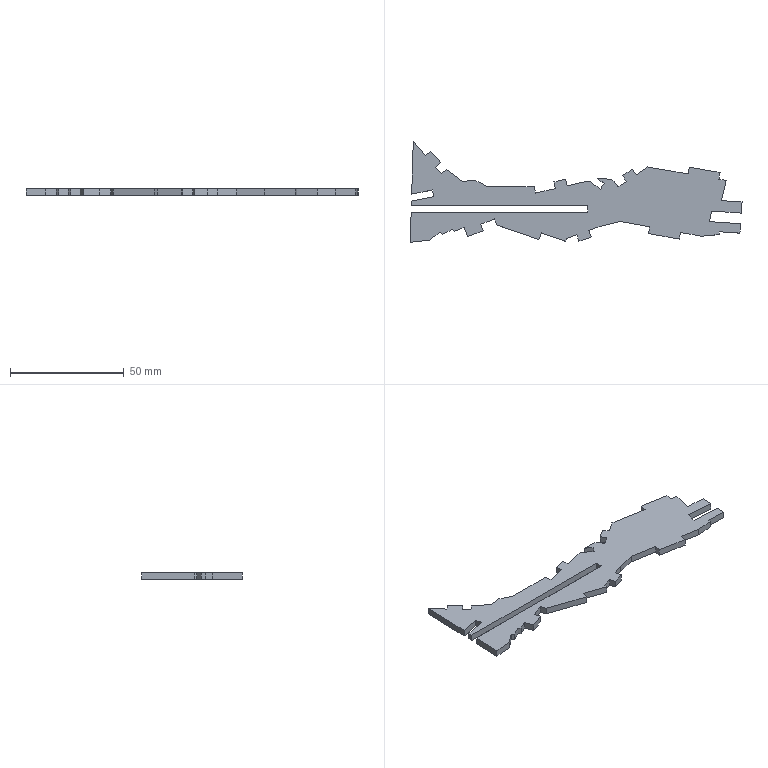Part | SolidWorks | features BaseBody 1 | 1 solid | 80 faces | box 146.238 x 44.263 x 3 mm | volume 9488 mm3 | plane 80